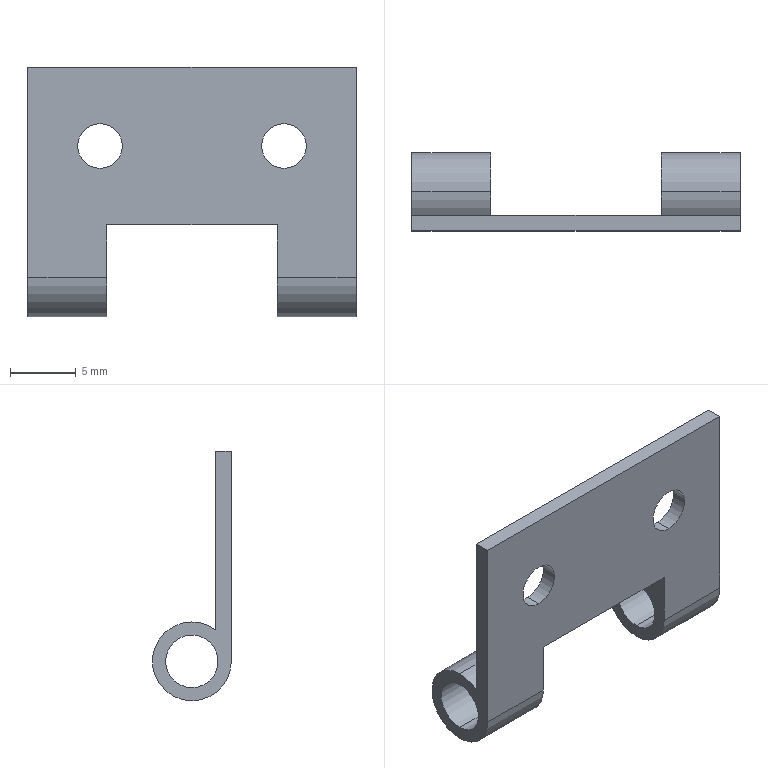Part | SolidWorks | features ICE 2, Extrusion 1 | 1 solid | 22 faces | box 25 x 6 x 19 mm | volume 560.152 mm3 | cylinder 14 | plane 8 | commonest cylinder face diameters 6 x6 3.4 x4 4 x4
STEP:
#1=CARTESIAN_POINT('',(-7.,-3.,8.3));
#2=VERTEX_POINT('',#1);
#3=CARTESIAN_POINT('',(-7.,-3.,11.7));
#4=VERTEX_POINT('',#3);
#5=CARTESIAN_POINT('',(-7.,-3.,10.));
#6=DIRECTION('',(0.,1.,0.));
#7=DIRECTION('',(0.,0.,1.));
#8=AXIS2_PLACEMENT_3D('',#5,#6,#7);
#9=CIRCLE('',#8,1.7);
#10=EDGE_CURVE('',#2,#4,#9,.T.);
#11=ORIENTED_EDGE('',*,*,#10,.F.);
#12=CARTESIAN_POINT('',(-7.,-1.8,8.3));
#13=VERTEX_POINT('',#12);
#14=CARTESIAN_POINT('',(-7.,-3.,8.3));
#15=DIRECTION('',(0.,1.,0.));
#16=VECTOR('',#15,1000.);
#17=LINE('',#14,#16);
#18=EDGE_CURVE('',#2,#13,#17,.T.);
#19=ORIENTED_EDGE('',*,*,#18,.T.);
#20=CARTESIAN_POINT('',(-7.,-1.8,11.7));
#21=VERTEX_POINT('',#20);
#22=CARTESIAN_POINT('',(-7.,-1.8,10.));
#23=DIRECTION('',(0.,1.,0.));
#24=DIRECTION('',(0.,0.,1.));
#25=AXIS2_PLACEMENT_3D('',#22,#23,#24);
#26=CIRCLE('',#25,1.7);
#27=EDGE_CURVE('',#13,#21,#26,.T.);
#28=ORIENTED_EDGE('',*,*,#27,.T.);
#29=CARTESIAN_POINT('',(-7.,-3.,11.7));
#30=DIRECTION('',(0.,1.,0.));
#31=VECTOR('',#30,1000.);
#32=LINE('',#29,#31);
#33=EDGE_CURVE('',#4,#21,#32,.T.);
#34=ORIENTED_EDGE('',*,*,#33,.F.);
#35=EDGE_LOOP('',(#11,#19,#28,#34));
#36=FACE_OUTER_BOUND('',#35,.T.);
#37=CARTESIAN_POINT('',(-7.,-3.,10.));
#38=DIRECTION('',(0.,1.,0.));
#39=DIRECTION('',(0.,0.,1.));
#40=AXIS2_PLACEMENT_3D('',#37,#38,#39);
#41=CYLINDRICAL_SURFACE('',#40,1.7);
#42=ADVANCED_FACE('',(#36),#41,.F.);
#43=CARTESIAN_POINT('',(7.,-3.,8.3));
#44=VERTEX_POINT('',#43);
#45=CARTESIAN_POINT('',(7.,-3.,11.7));
#46=VERTEX_POINT('',#45);
#47=CARTESIAN_POINT('',(7.,-3.,10.));
#48=DIRECTION('',(0.,1.,0.));
#49=DIRECTION('',(0.,0.,1.));
#50=AXIS2_PLACEMENT_3D('',#47,#48,#49);
#51=CIRCLE('',#50,1.7);
#52=EDGE_CURVE('',#44,#46,#51,.T.);
#53=ORIENTED_EDGE('',*,*,#52,.F.);
#54=CARTESIAN_POINT('',(7.,-1.8,8.3));
#55=VERTEX_POINT('',#54);
#56=CARTESIAN_POINT('',(7.,-3.,8.3));
#57=DIRECTION('',(0.,1.,0.));
#58=VECTOR('',#57,1000.);
#59=LINE('',#56,#58);
#60=EDGE_CURVE('',#44,#55,#59,.T.);
#61=ORIENTED_EDGE('',*,*,#60,.T.);
#62=CARTESIAN_POINT('',(7.,-1.8,11.7));
#63=VERTEX_POINT('',#62);
#64=CARTESIAN_POINT('',(7.,-1.8,10.));
#65=DIRECTION('',(0.,1.,0.));
#66=DIRECTION('',(0.,0.,1.));
#67=AXIS2_PLACEMENT_3D('',#64,#65,#66);
#68=CIRCLE('',#67,1.7);
#69=EDGE_CURVE('',#55,#63,#68,.T.);
#70=ORIENTED_EDGE('',*,*,#69,.T.);
#71=CARTESIAN_POINT('',(7.,-3.,11.7));
#72=DIRECTION('',(0.,1.,0.));
#73=VECTOR('',#72,1000.);
#74=LINE('',#71,#73);
#75=EDGE_CURVE('',#46,#63,#74,.T.);
#76=ORIENTED_EDGE('',*,*,#75,.F.);
#77=EDGE_LOOP('',(#53,#61,#70,#76));
#78=FACE_OUTER_BOUND('',#77,.T.);
#79=CARTESIAN_POINT('',(7.,-3.,10.));
#80=DIRECTION('',(0.,1.,0.));
#81=DIRECTION('',(0.,0.,1.));
#82=AXIS2_PLACEMENT_3D('',#79,#80,#81);
#83=CYLINDRICAL_SURFACE('',#82,1.7);
#84=ADVANCED_FACE('',(#78),#83,.F.);
#85=CARTESIAN_POINT('',(12.5,0.,2.));
#86=VERTEX_POINT('',#85);
#87=CARTESIAN_POINT('',(12.5,0.,-2.));
#88=VERTEX_POINT('',#87);
#89=CARTESIAN_POINT('',(12.5,0.,0.));
#90=DIRECTION('',(1.,0.,0.));
#91=DIRECTION('',(0.,0.,-1.));
#92=AXIS2_PLACEMENT_3D('',#89,#90,#91);
#93=CIRCLE('',#92,2.);
#94=EDGE_CURVE('',#86,#88,#93,.T.);
#95=ORIENTED_EDGE('',*,*,#94,.T.);
#96=CARTESIAN_POINT('',(6.5,0.,-2.));
#97=VERTEX_POINT('',#96);
#98=CARTESIAN_POINT('',(12.5,0.,-2.));
#99=DIRECTION('',(-1.,0.,0.));
#100=VECTOR('',#99,1000.);
#101=LINE('',#98,#100);
#102=EDGE_CURVE('',#88,#97,#101,.T.);
#103=ORIENTED_EDGE('',*,*,#102,.T.);
#104=CARTESIAN_POINT('',(6.5,0.,2.));
#105=VERTEX_POINT('',#104);
#106=CARTESIAN_POINT('',(6.5,0.,0.));
#107=DIRECTION('',(1.,0.,0.));
#108=DIRECTION('',(0.,0.,-1.));
#109=AXIS2_PLACEMENT_3D('',#106,#107,#108);
#110=CIRCLE('',#109,2.);
#111=EDGE_CURVE('',#105,#97,#110,.T.);
#112=ORIENTED_EDGE('',*,*,#111,.F.);
#113=CARTESIAN_POINT('',(12.5,0.,2.));
#114=DIRECTION('',(-1.,0.,0.));
#115=VECTOR('',#114,1000.);
#116=LINE('',#113,#115);
#117=EDGE_CURVE('',#86,#105,#116,.T.);
#118=ORIENTED_EDGE('',*,*,#117,.F.);
#119=EDGE_LOOP('',(#95,#103,#112,#118));
#120=FACE_OUTER_BOUND('',#119,.T.);
#121=CARTESIAN_POINT('',(12.5,0.,0.));
#122=DIRECTION('',(-1.,0.,0.));
#123=DIRECTION('',(0.,0.,1.));
#124=AXIS2_PLACEMENT_3D('',#121,#122,#123);
#125=CYLINDRICAL_SURFACE('',#124,2.);
#126=ADVANCED_FACE('',(#120),#125,.F.);
#127=CARTESIAN_POINT('',(12.5,0.,-3.));
#128=VERTEX_POINT('',#127);
#129=CARTESIAN_POINT('',(12.5,0.,3.));
#130=VERTEX_POINT('',#129);
#131=CARTESIAN_POINT('',(12.5,0.,0.));
#132=DIRECTION('',(1.,0.,0.));
#133=DIRECTION('',(0.,0.,-1.));
#134=AXIS2_PLACEMENT_3D('',#131,#132,#133);
#135=CIRCLE('',#134,3.);
#136=EDGE_CURVE('',#128,#130,#135,.T.);
#137=ORIENTED_EDGE('',*,*,#136,.F.);
#138=CARTESIAN_POINT('',(6.5,0.,-3.));
#139=VERTEX_POINT('',#138);
#140=CARTESIAN_POINT('',(12.5,0.,-3.));
#141=DIRECTION('',(-1.,0.,0.));
#142=VECTOR('',#141,1000.);
#143=LINE('',#140,#142);
#144=EDGE_CURVE('',#128,#139,#143,.T.);
#145=ORIENTED_EDGE('',*,*,#144,.T.);
#146=CARTESIAN_POINT('',(6.5,0.,3.));
#147=VERTEX_POINT('',#146);
#148=CARTESIAN_POINT('',(6.5,0.,0.));
#149=DIRECTION('',(1.,0.,0.));
#150=DIRECTION('',(0.,0.,-1.));
#151=AXIS2_PLACEMENT_3D('',#148,#149,#150);
#152=CIRCLE('',#151,3.);
#153=EDGE_CURVE('',#139,#147,#152,.T.);
#154=ORIENTED_EDGE('',*,*,#153,.T.);
#155=CARTESIAN_POINT('',(12.5,0.,3.));
#156=DIRECTION('',(-1.,0.,0.));
#157=VECTOR('',#156,1000.);
#158=LINE('',#155,#157);
#159=EDGE_CURVE('',#130,#147,#158,.T.);
#160=ORIENTED_EDGE('',*,*,#159,.F.);
#161=EDGE_LOOP('',(#137,#145,#154,#160));
#162=FACE_OUTER_BOUND('',#161,.T.);
#163=CARTESIAN_POINT('',(12.5,0.,0.));
#164=DIRECTION('',(-1.,0.,0.));
#165=DIRECTION('',(0.,0.,1.));
#166=AXIS2_PLACEMENT_3D('',#163,#164,#165);
#167=CYLINDRICAL_SURFACE('',#166,3.);
#168=ADVANCED_FACE('',(#162),#167,.T.);
#169=CARTESIAN_POINT('',(12.5,-1.8,2.4));
#170=VERTEX_POINT('',#169);
#171=CARTESIAN_POINT('',(12.5,0.,0.));
#172=DIRECTION('',(1.,0.,0.));
#173=DIRECTION('',(0.,0.,-1.));
#174=AXIS2_PLACEMENT_3D('',#171,#172,#173);
#175=CIRCLE('',#174,3.);
#176=EDGE_CURVE('',#130,#170,#175,.T.);
#177=ORIENTED_EDGE('',*,*,#176,.F.);
#178=ORIENTED_EDGE('',*,*,#159,.T.);
#179=CARTESIAN_POINT('',(6.5,-1.8,2.4));
#180=VERTEX_POINT('',#179);
#181=CARTESIAN_POINT('',(6.5,0.,0.));
#182=DIRECTION('',(1.,0.,0.));
#183=DIRECTION('',(0.,0.,-1.));
#184=AXIS2_PLACEMENT_3D('',#181,#182,#183);
#185=CIRCLE('',#184,3.);
#186=EDGE_CURVE('',#147,#180,#185,.T.);
#187=ORIENTED_EDGE('',*,*,#186,.T.);
#188=CARTESIAN_POINT('',(12.5,-1.8,2.4));
#189=DIRECTION('',(-1.,0.,0.));
#190=VECTOR('',#189,1000.);
#191=LINE('',#188,#190);
#192=EDGE_CURVE('',#170,#180,#191,.T.);
#193=ORIENTED_EDGE('',*,*,#192,.F.);
#194=EDGE_LOOP('',(#177,#178,#187,#193));
#195=FACE_OUTER_BOUND('',#194,.T.);
#196=CARTESIAN_POINT('',(12.5,0.,0.));
#197=DIRECTION('',(-1.,0.,0.));
#198=DIRECTION('',(0.,0.,1.));
#199=AXIS2_PLACEMENT_3D('',#196,#197,#198);
#200=CYLINDRICAL_SURFACE('',#199,3.);
#201=ADVANCED_FACE('',(#195),#200,.T.);
#202=CARTESIAN_POINT('',(-6.5,0.,2.));
#203=VERTEX_POINT('',#202);
#204=CARTESIAN_POINT('',(-6.5,0.,-2.));
#205=VERTEX_POINT('',#204);
#206=CARTESIAN_POINT('',(-6.5,0.,0.));
#207=DIRECTION('',(1.,0.,0.));
#208=DIRECTION('',(0.,0.,-1.));
#209=AXIS2_PLACEMENT_3D('',#206,#207,#208);
#210=CIRCLE('',#209,2.);
#211=EDGE_CURVE('',#203,#205,#210,.T.);
#212=ORIENTED_EDGE('',*,*,#211,.T.);
#213=CARTESIAN_POINT('',(-12.5,0.,-2.));
#214=VERTEX_POINT('',#213);
#215=CARTESIAN_POINT('',(12.5,0.,-2.));
#216=DIRECTION('',(-1.,0.,0.));
#217=VECTOR('',#216,1000.);
#218=LINE('',#215,#217);
#219=EDGE_CURVE('',#205,#214,#218,.T.);
#220=ORIENTED_EDGE('',*,*,#219,.T.);
#221=CARTESIAN_POINT('',(-12.5,0.,2.));
#222=VERTEX_POINT('',#221);
#223=CARTESIAN_POINT('',(-12.5,0.,0.));
#224=DIRECTION('',(1.,0.,0.));
#225=DIRECTION('',(0.,0.,-1.));
#226=AXIS2_PLACEMENT_3D('',#223,#224,#225);
#227=CIRCLE('',#226,2.);
#228=EDGE_CURVE('',#222,#214,#227,.T.);
#229=ORIENTED_EDGE('',*,*,#228,.F.);
#230=CARTESIAN_POINT('',(12.5,0.,2.));
#231=DIRECTION('',(-1.,0.,0.));
#232=VECTOR('',#231,1000.);
#233=LINE('',#230,#232);
#234=EDGE_CURVE('',#203,#222,#233,.T.);
#235=ORIENTED_EDGE('',*,*,#234,.F.);
#236=EDGE_LOOP('',(#212,#220,#229,#235));
#237=FACE_OUTER_BOUND('',#236,.T.);
#238=CARTESIAN_POINT('',(12.5,0.,0.));
#239=DIRECTION('',(-1.,0.,0.));
#240=DIRECTION('',(0.,0.,1.));
#241=AXIS2_PLACEMENT_3D('',#238,#239,#240);
#242=CYLINDRICAL_SURFACE('',#241,2.);
#243=ADVANCED_FACE('',(#237),#242,.F.);
#244=CARTESIAN_POINT('',(-6.5,0.,-3.));
#245=VERTEX_POINT('',#244);
#246=CARTESIAN_POINT('',(-6.5,0.,3.));
#247=VERTEX_POINT('',#246);
#248=CARTESIAN_POINT('',(-6.5,0.,0.));
#249=DIRECTION('',(1.,0.,0.));
#250=DIRECTION('',(0.,0.,-1.));
#251=AXIS2_PLACEMENT_3D('',#248,#249,#250);
#252=CIRCLE('',#251,3.);
#253=EDGE_CURVE('',#245,#247,#252,.T.);
#254=ORIENTED_EDGE('',*,*,#253,.F.);
#255=CARTESIAN_POINT('',(-12.5,0.,-3.));
#256=VERTEX_POINT('',#255);
#257=CARTESIAN_POINT('',(12.5,0.,-3.));
#258=DIRECTION('',(-1.,0.,0.));
#259=VECTOR('',#258,1000.);
#260=LINE('',#257,#259);
#261=EDGE_CURVE('',#245,#256,#260,.T.);
#262=ORIENTED_EDGE('',*,*,#261,.T.);
#263=CARTESIAN_POINT('',(-12.5,0.,3.));
#264=VERTEX_POINT('',#263);
#265=CARTESIAN_POINT('',(-12.5,0.,0.));
#266=DIRECTION('',(1.,0.,0.));
#267=DIRECTION('',(0.,0.,-1.));
#268=AXIS2_PLACEMENT_3D('',#265,#266,#267);
#269=CIRCLE('',#268,3.);
#270=EDGE_CURVE('',#256,#264,#269,.T.);
#271=ORIENTED_EDGE('',*,*,#270,.T.);
#272=CARTESIAN_POINT('',(12.5,0.,3.));
#273=DIRECTION('',(-1.,0.,0.));
#274=VECTOR('',#273,1000.);
#275=LINE('',#272,#274);
#276=EDGE_CURVE('',#247,#264,#275,.T.);
#277=ORIENTED_EDGE('',*,*,#276,.F.);
#278=EDGE_LOOP('',(#254,#262,#271,#277));
#279=FACE_OUTER_BOUND('',#278,.T.);
#280=CARTESIAN_POINT('',(12.5,0.,0.));
#281=DIRECTION('',(-1.,0.,0.));
#282=DIRECTION('',(0.,0.,1.));
#283=AXIS2_PLACEMENT_3D('',#280,#281,#282);
#284=CYLINDRICAL_SURFACE('',#283,3.);
#285=ADVANCED_FACE('',(#279),#284,.T.);
#286=CARTESIAN_POINT('',(-6.5,-1.8,2.4));
#287=VERTEX_POINT('',#286);
#288=CARTESIAN_POINT('',(-6.5,0.,0.));
#289=DIRECTION('',(1.,0.,0.));
#290=DIRECTION('',(0.,0.,-1.));
#291=AXIS2_PLACEMENT_3D('',#288,#289,#290);
#292=CIRCLE('',#291,3.);
#293=EDGE_CURVE('',#247,#287,#292,.T.);
#294=ORIENTED_EDGE('',*,*,#293,.F.);
#295=ORIENTED_EDGE('',*,*,#276,.T.);
#296=CARTESIAN_POINT('',(-12.5,-1.8,2.4));
#297=VERTEX_POINT('',#296);
#298=CARTESIAN_POINT('',(-12.5,0.,0.));
#299=DIRECTION('',(1.,0.,0.));
#300=DIRECTION('',(0.,0.,-1.));
#301=AXIS2_PLACEMENT_3D('',#298,#299,#300);
#302=CIRCLE('',#301,3.);
#303=EDGE_CURVE('',#264,#297,#302,.T.);
#304=ORIENTED_EDGE('',*,*,#303,.T.);
#305=CARTESIAN_POINT('',(12.5,-1.8,2.4));
#306=DIRECTION('',(-1.,0.,0.));
#307=VECTOR('',#306,1000.);
#308=LINE('',#305,#307);
#309=EDGE_CURVE('',#287,#297,#308,.T.);
#310=ORIENTED_EDGE('',*,*,#309,.F.);
#311=EDGE_LOOP('',(#294,#295,#304,#310));
#312=FACE_OUTER_BOUND('',#311,.T.);
#313=CARTESIAN_POINT('',(12.5,0.,0.));
#314=DIRECTION('',(-1.,0.,0.));
#315=DIRECTION('',(0.,0.,1.));
#316=AXIS2_PLACEMENT_3D('',#313,#314,#315);
#317=CYLINDRICAL_SURFACE('',#316,3.);
#318=ADVANCED_FACE('',(#312),#317,.T.);
#319=ORIENTED_EDGE('',*,*,#261,.F.);
#320=CARTESIAN_POINT('',(-6.5,-3.,0.));
#321=VERTEX_POINT('',#320);
#322=CARTESIAN_POINT('',(-6.5,0.,0.));
#323=DIRECTION('',(1.,0.,0.));
#324=DIRECTION('',(0.,0.,-1.));
#325=AXIS2_PLACEMENT_3D('',#322,#323,#324);
#326=CIRCLE('',#325,3.);
#327=EDGE_CURVE('',#321,#245,#326,.T.);
#328=ORIENTED_EDGE('',*,*,#327,.F.);
#329=CARTESIAN_POINT('',(-12.5,-3.,0.));
#330=VERTEX_POINT('',#329);
#331=CARTESIAN_POINT('',(12.5,-3.,0.));
#332=DIRECTION('',(-1.,0.,0.));
#333=VECTOR('',#332,1000.);
#334=LINE('',#331,#333);
#335=EDGE_CURVE('',#321,#330,#334,.T.);
#336=ORIENTED_EDGE('',*,*,#335,.T.);
#337=CARTESIAN_POINT('',(-12.5,0.,0.));
#338=DIRECTION('',(1.,0.,0.));
#339=DIRECTION('',(0.,0.,-1.));
#340=AXIS2_PLACEMENT_3D('',#337,#338,#339);
#341=CIRCLE('',#340,3.);
#342=EDGE_CURVE('',#330,#256,#341,.T.);
#343=ORIENTED_EDGE('',*,*,#342,.T.);
#344=EDGE_LOOP('',(#319,#328,#336,#343));
#345=FACE_OUTER_BOUND('',#344,.T.);
#346=CARTESIAN_POINT('',(12.5,0.,0.));
#347=DIRECTION('',(-1.,0.,0.));
#348=DIRECTION('',(0.,0.,1.));
#349=AXIS2_PLACEMENT_3D('',#346,#347,#348);
#350=CYLINDRICAL_SURFACE('',#349,3.);
#351=ADVANCED_FACE('',(#345),#350,.T.);
#352=CARTESIAN_POINT('',(7.,-1.8,10.));
#353=DIRECTION('',(0.,1.,0.));
#354=DIRECTION('',(0.,0.,1.));
#355=AXIS2_PLACEMENT_3D('',#352,#353,#354);
#356=CIRCLE('',#355,1.7);
#357=EDGE_CURVE('',#63,#55,#356,.T.);
#358=ORIENTED_EDGE('',*,*,#357,.F.);
#359=ORIENTED_EDGE('',*,*,#69,.F.);
#360=EDGE_LOOP('',(#358,#359));
#361=FACE_BOUND('',#360,.T.);
#362=CARTESIAN_POINT('',(-7.,-1.8,10.));
#363=DIRECTION('',(0.,1.,0.));
#364=DIRECTION('',(0.,0.,1.));
#365=AXIS2_PLACEMENT_3D('',#362,#363,#364);
#366=CIRCLE('',#365,1.7);
#367=EDGE_CURVE('',#21,#13,#366,.T.);
#368=ORIENTED_EDGE('',*,*,#367,.F.);
#369=ORIENTED_EDGE('',*,*,#27,.F.);
#370=EDGE_LOOP('',(#368,#369));
#371=FACE_BOUND('',#370,.T.);
#372=CARTESIAN_POINT('',(-6.5,-1.8,4.));
#373=VERTEX_POINT('',#372);
#374=CARTESIAN_POINT('',(-6.5,-1.8,2.4));
#375=DIRECTION('',(0.,0.,1.));
#376=VECTOR('',#375,1000.);
#377=LINE('',#374,#376);
#378=EDGE_CURVE('',#287,#373,#377,.T.);
#379=ORIENTED_EDGE('',*,*,#378,.F.);
#380=ORIENTED_EDGE('',*,*,#309,.T.);
#381=CARTESIAN_POINT('',(-12.5,-1.8,16.));
#382=VERTEX_POINT('',#381);
#383=CARTESIAN_POINT('',(-12.5,-1.8,16.));
#384=DIRECTION('',(0.,0.,1.));
#385=VECTOR('',#384,1000.);
#386=LINE('',#383,#385);
#387=EDGE_CURVE('',#297,#382,#386,.T.);
#388=ORIENTED_EDGE('',*,*,#387,.T.);
#389=CARTESIAN_POINT('',(12.5,-1.8,16.));
#390=VERTEX_POINT('',#389);
#391=CARTESIAN_POINT('',(12.5,-1.8,16.));
#392=DIRECTION('',(-1.,0.,0.));
#393=VECTOR('',#392,1000.);
#394=LINE('',#391,#393);
#395=EDGE_CURVE('',#390,#382,#394,.T.);
#396=ORIENTED_EDGE('',*,*,#395,.F.);
#397=CARTESIAN_POINT('',(12.5,-1.8,16.));
#398=DIRECTION('',(0.,0.,1.));
#399=VECTOR('',#398,1000.);
#400=LINE('',#397,#399);
#401=EDGE_CURVE('',#170,#390,#400,.T.);
#402=ORIENTED_EDGE('',*,*,#401,.F.);
#403=ORIENTED_EDGE('',*,*,#192,.T.);
#404=CARTESIAN_POINT('',(6.5,-1.8,4.));
#405=VERTEX_POINT('',#404);
#406=CARTESIAN_POINT('',(6.5,-1.8,2.4));
#407=DIRECTION('',(0.,0.,1.));
#408=VECTOR('',#407,1000.);
#409=LINE('',#406,#408);
#410=EDGE_CURVE('',#180,#405,#409,.T.);
#411=ORIENTED_EDGE('',*,*,#410,.T.);
#412=CARTESIAN_POINT('',(-6.5,-1.8,4.));
#413=DIRECTION('',(1.,0.,0.));
#414=VECTOR('',#413,1000.);
#415=LINE('',#412,#414);
#416=EDGE_CURVE('',#373,#405,#415,.T.);
#417=ORIENTED_EDGE('',*,*,#416,.F.);
#418=EDGE_LOOP('',(#379,#380,#388,#396,#402,#403,#411,#417));
#419=FACE_OUTER_BOUND('',#418,.T.);
#420=CARTESIAN_POINT('',(12.5,-1.8,16.));
#421=DIRECTION('',(0.,-1.,0.));
#422=DIRECTION('',(0.,0.,-1.));
#423=AXIS2_PLACEMENT_3D('',#420,#421,#422);
#424=PLANE('',#423);
#425=ADVANCED_FACE('',(#361,#371,#419),#424,.F.);
#426=CARTESIAN_POINT('',(7.,-3.,10.));
#427=DIRECTION('',(0.,1.,0.));
#428=DIRECTION('',(0.,0.,1.));
#429=AXIS2_PLACEMENT_3D('',#426,#427,#428);
#430=CIRCLE('',#429,1.7);
#431=EDGE_CURVE('',#46,#44,#430,.T.);
#432=ORIENTED_EDGE('',*,*,#431,.T.);
#433=ORIENTED_EDGE('',*,*,#52,.T.);
#434=EDGE_LOOP('',(#432,#433));
#435=FACE_BOUND('',#434,.T.);
#436=CARTESIAN_POINT('',(-7.,-3.,10.));
#437=DIRECTION('',(0.,1.,0.));
#438=DIRECTION('',(0.,0.,1.));
#439=AXIS2_PLACEMENT_3D('',#436,#437,#438);
#440=CIRCLE('',#439,1.7);
#441=EDGE_CURVE('',#4,#2,#440,.T.);
#442=ORIENTED_EDGE('',*,*,#441,.T.);
#443=ORIENTED_EDGE('',*,*,#10,.T.);
#444=EDGE_LOOP('',(#442,#443));
#445=FACE_BOUND('',#444,.T.);
#446=CARTESIAN_POINT('',(-6.5,-3.,4.));
#447=VERTEX_POINT('',#446);
#448=CARTESIAN_POINT('',(-6.5,-3.,4.));
#449=DIRECTION('',(0.,0.,-1.));
#450=VECTOR('',#449,1000.);
#451=LINE('',#448,#450);
#452=EDGE_CURVE('',#447,#321,#451,.T.);
#453=ORIENTED_EDGE('',*,*,#452,.F.);
#454=CARTESIAN_POINT('',(6.5,-3.,4.));
#455=VERTEX_POINT('',#454);
#456=CARTESIAN_POINT('',(-6.5,-3.,4.));
#457=DIRECTION('',(1.,0.,0.));
#458=VECTOR('',#457,1000.);
#459=LINE('',#456,#458);
#460=EDGE_CURVE('',#447,#455,#459,.T.);
#461=ORIENTED_EDGE('',*,*,#460,.T.);
#462=CARTESIAN_POINT('',(6.5,-3.,0.));
#463=VERTEX_POINT('',#462);
#464=CARTESIAN_POINT('',(6.5,-3.,4.));
#465=DIRECTION('',(0.,0.,-1.));
#466=VECTOR('',#465,1000.);
#467=LINE('',#464,#466);
#468=EDGE_CURVE('',#455,#463,#467,.T.);
#469=ORIENTED_EDGE('',*,*,#468,.T.);
#470=CARTESIAN_POINT('',(12.5,-3.,0.));
#471=VERTEX_POINT('',#470);
#472=CARTESIAN_POINT('',(12.5,-3.,0.));
#473=DIRECTION('',(-1.,0.,0.));
#474=VECTOR('',#473,1000.);
#475=LINE('',#472,#474);
#476=EDGE_CURVE('',#471,#463,#475,.T.);
#477=ORIENTED_EDGE('',*,*,#476,.F.);
#478=CARTESIAN_POINT('',(12.5,-3.,16.));
#479=VERTEX_POINT('',#478);
#480=CARTESIAN_POINT('',(12.5,-3.,0.));
#481=DIRECTION('',(0.,0.,-1.));
#482=VECTOR('',#481,1000.);
#483=LINE('',#480,#482);
#484=EDGE_CURVE('',#479,#471,#483,.T.);
#485=ORIENTED_EDGE('',*,*,#484,.F.);
#486=CARTESIAN_POINT('',(-12.5,-3.,16.));
#487=VERTEX_POINT('',#486);
#488=CARTESIAN_POINT('',(12.5,-3.,16.));
#489=DIRECTION('',(-1.,0.,0.));
#490=VECTOR('',#489,1000.);
#491=LINE('',#488,#490);
#492=EDGE_CURVE('',#479,#487,#491,.T.);
#493=ORIENTED_EDGE('',*,*,#492,.T.);
#494=CARTESIAN_POINT('',(-12.5,-3.,0.));
#495=DIRECTION('',(0.,0.,-1.));
#496=VECTOR('',#495,1000.);
#497=LINE('',#494,#496);
#498=EDGE_CURVE('',#487,#330,#497,.T.);
#499=ORIENTED_EDGE('',*,*,#498,.T.);
#500=ORIENTED_EDGE('',*,*,#335,.F.);
#501=EDGE_LOOP('',(#453,#461,#469,#477,#485,#493,#499,#500));
#502=FACE_OUTER_BOUND('',#501,.T.);
#503=CARTESIAN_POINT('',(12.5,-3.,0.));
#504=DIRECTION('',(0.,1.,0.));
#505=DIRECTION('',(0.,0.,1.));
#506=AXIS2_PLACEMENT_3D('',#503,#504,#505);
#507=PLANE('',#506);
#508=ADVANCED_FACE('',(#435,#445,#502),#507,.F.);
#509=ORIENTED_EDGE('',*,*,#219,.F.);
#510=CARTESIAN_POINT('',(-6.5,0.,0.));
#511=DIRECTION('',(1.,0.,0.));
#512=DIRECTION('',(0.,0.,-1.));
#513=AXIS2_PLACEMENT_3D('',#510,#511,#512);
#514=CIRCLE('',#513,2.);
#515=EDGE_CURVE('',#205,#203,#514,.T.);
#516=ORIENTED_EDGE('',*,*,#515,.T.);
#517=ORIENTED_EDGE('',*,*,#234,.T.);
#518=CARTESIAN_POINT('',(-12.5,0.,0.));
#519=DIRECTION('',(1.,0.,0.));
#520=DIRECTION('',(0.,0.,-1.));
#521=AXIS2_PLACEMENT_3D('',#518,#519,#520);
#522=CIRCLE('',#521,2.);
#523=EDGE_CURVE('',#214,#222,#522,.T.);
#524=ORIENTED_EDGE('',*,*,#523,.F.);
#525=EDGE_LOOP('',(#509,#516,#517,#524));
#526=FACE_OUTER_BOUND('',#525,.T.);
#527=CARTESIAN_POINT('',(12.5,0.,0.));
#528=DIRECTION('',(-1.,0.,0.));
#529=DIRECTION('',(0.,0.,1.));
#530=AXIS2_PLACEMENT_3D('',#527,#528,#529);
#531=CYLINDRICAL_SURFACE('',#530,2.);
#532=ADVANCED_FACE('',(#526),#531,.F.);
#533=CARTESIAN_POINT('',(12.5,0.,0.));
#534=DIRECTION('',(1.,0.,0.));
#535=DIRECTION('',(0.,0.,-1.));
#536=AXIS2_PLACEMENT_3D('',#533,#534,#535);
#537=CIRCLE('',#536,3.);
#538=EDGE_CURVE('',#471,#128,#537,.T.);
#539=ORIENTED_EDGE('',*,*,#538,.T.);
#540=ORIENTED_EDGE('',*,*,#136,.T.);
#541=ORIENTED_EDGE('',*,*,#176,.T.);
#542=ORIENTED_EDGE('',*,*,#401,.T.);
#543=CARTESIAN_POINT('',(12.5,-3.,16.));
#544=DIRECTION('',(0.,-1.,0.));
#545=VECTOR('',#544,1000.);
#546=LINE('',#543,#545);
#547=EDGE_CURVE('',#390,#479,#546,.T.);
#548=ORIENTED_EDGE('',*,*,#547,.T.);
#549=ORIENTED_EDGE('',*,*,#484,.T.);
#550=EDGE_LOOP('',(#539,#540,#541,#542,#548,#549));
#551=FACE_OUTER_BOUND('',#550,.T.);
#552=ORIENTED_EDGE('',*,*,#94,.F.);
#553=CARTESIAN_POINT('',(12.5,0.,0.));
#554=DIRECTION('',(1.,0.,0.));
#555=DIRECTION('',(0.,0.,-1.));
#556=AXIS2_PLACEMENT_3D('',#553,#554,#555);
#557=CIRCLE('',#556,2.);
#558=EDGE_CURVE('',#88,#86,#557,.T.);
#559=ORIENTED_EDGE('',*,*,#558,.F.);
#560=EDGE_LOOP('',(#552,#559));
#561=FACE_BOUND('',#560,.T.);
#562=CARTESIAN_POINT('',(12.5,0.,0.));
#563=DIRECTION('',(1.,0.,0.));
#564=DIRECTION('',(0.,0.,-1.));
#565=AXIS2_PLACEMENT_3D('',#562,#563,#564);
#566=PLANE('',#565);
#567=ADVANCED_FACE('',(#551,#561),#566,.T.);
#568=ORIENTED_EDGE('',*,*,#342,.F.);
#569=ORIENTED_EDGE('',*,*,#498,.F.);
#570=CARTESIAN_POINT('',(-12.5,-3.,16.));
#571=DIRECTION('',(0.,-1.,0.));
#572=VECTOR('',#571,1000.);
#573=LINE('',#570,#572);
#574=EDGE_CURVE('',#382,#487,#573,.T.);
#575=ORIENTED_EDGE('',*,*,#574,.F.);
#576=ORIENTED_EDGE('',*,*,#387,.F.);
#577=ORIENTED_EDGE('',*,*,#303,.F.);
#578=ORIENTED_EDGE('',*,*,#270,.F.);
#579=EDGE_LOOP('',(#568,#569,#575,#576,#577,#578));
#580=FACE_OUTER_BOUND('',#579,.T.);
#581=ORIENTED_EDGE('',*,*,#228,.T.);
#582=ORIENTED_EDGE('',*,*,#523,.T.);
#583=EDGE_LOOP('',(#581,#582));
#584=FACE_BOUND('',#583,.T.);
#585=CARTESIAN_POINT('',(-12.5,0.,0.));
#586=DIRECTION('',(1.,0.,0.));
#587=DIRECTION('',(0.,0.,-1.));
#588=AXIS2_PLACEMENT_3D('',#585,#586,#587);
#589=PLANE('',#588);
#590=ADVANCED_FACE('',(#580,#584),#589,.F.);
#591=ORIENTED_EDGE('',*,*,#144,.F.);
#592=ORIENTED_EDGE('',*,*,#538,.F.);
#593=ORIENTED_EDGE('',*,*,#476,.T.);
#594=CARTESIAN_POINT('',(6.5,0.,0.));
#595=DIRECTION('',(1.,0.,0.));
#596=DIRECTION('',(0.,0.,-1.));
#597=AXIS2_PLACEMENT_3D('',#594,#595,#596);
#598=CIRCLE('',#597,3.);
#599=EDGE_CURVE('',#463,#139,#598,.T.);
#600=ORIENTED_EDGE('',*,*,#599,.T.);
#601=EDGE_LOOP('',(#591,#592,#593,#600));
#602=FACE_OUTER_BOUND('',#601,.T.);
#603=CARTESIAN_POINT('',(12.5,0.,0.));
#604=DIRECTION('',(-1.,0.,0.));
#605=DIRECTION('',(0.,0.,1.));
#606=AXIS2_PLACEMENT_3D('',#603,#604,#605);
#607=CYLINDRICAL_SURFACE('',#606,3.);
#608=ADVANCED_FACE('',(#602),#607,.T.);
#609=ORIENTED_EDGE('',*,*,#574,.T.);
#610=ORIENTED_EDGE('',*,*,#492,.F.);
#611=ORIENTED_EDGE('',*,*,#547,.F.);
#612=ORIENTED_EDGE('',*,*,#395,.T.);
#613=EDGE_LOOP('',(#609,#610,#611,#612));
#614=FACE_OUTER_BOUND('',#613,.T.);
#615=CARTESIAN_POINT('',(12.5,-3.,16.));
#616=DIRECTION('',(0.,0.,-1.));
#617=DIRECTION('',(-1.,0.,0.));
#618=AXIS2_PLACEMENT_3D('',#615,#616,#617);
#619=PLANE('',#618);
#620=ADVANCED_FACE('',(#614),#619,.F.);
#621=ORIENTED_EDGE('',*,*,#102,.F.);
#622=ORIENTED_EDGE('',*,*,#558,.T.);
#623=ORIENTED_EDGE('',*,*,#117,.T.);
#624=CARTESIAN_POINT('',(6.5,0.,0.));
#625=DIRECTION('',(1.,0.,0.));
#626=DIRECTION('',(0.,0.,-1.));
#627=AXIS2_PLACEMENT_3D('',#624,#625,#626);
#628=CIRCLE('',#627,2.);
#629=EDGE_CURVE('',#97,#105,#628,.T.);
#630=ORIENTED_EDGE('',*,*,#629,.F.);
#631=EDGE_LOOP('',(#621,#622,#623,#630));
#632=FACE_OUTER_BOUND('',#631,.T.);
#633=CARTESIAN_POINT('',(12.5,0.,0.));
#634=DIRECTION('',(-1.,0.,0.));
#635=DIRECTION('',(0.,0.,1.));
#636=AXIS2_PLACEMENT_3D('',#633,#634,#635);
#637=CYLINDRICAL_SURFACE('',#636,2.);
#638=ADVANCED_FACE('',(#632),#637,.F.);
#639=ORIENTED_EDGE('',*,*,#60,.F.);
#640=ORIENTED_EDGE('',*,*,#431,.F.);
#641=ORIENTED_EDGE('',*,*,#75,.T.);
#642=ORIENTED_EDGE('',*,*,#357,.T.);
#643=EDGE_LOOP('',(#639,#640,#641,#642));
#644=FACE_OUTER_BOUND('',#643,.T.);
#645=CARTESIAN_POINT('',(7.,-3.,10.));
#646=DIRECTION('',(0.,1.,0.));
#647=DIRECTION('',(0.,0.,1.));
#648=AXIS2_PLACEMENT_3D('',#645,#646,#647);
#649=CYLINDRICAL_SURFACE('',#648,1.7);
#650=ADVANCED_FACE('',(#644),#649,.F.);
#651=ORIENTED_EDGE('',*,*,#18,.F.);
#652=ORIENTED_EDGE('',*,*,#441,.F.);
#653=ORIENTED_EDGE('',*,*,#33,.T.);
#654=ORIENTED_EDGE('',*,*,#367,.T.);
#655=EDGE_LOOP('',(#651,#652,#653,#654));
#656=FACE_OUTER_BOUND('',#655,.T.);
#657=CARTESIAN_POINT('',(-7.,-3.,10.));
#658=DIRECTION('',(0.,1.,0.));
#659=DIRECTION('',(0.,0.,1.));
#660=AXIS2_PLACEMENT_3D('',#657,#658,#659);
#661=CYLINDRICAL_SURFACE('',#660,1.7);
#662=ADVANCED_FACE('',(#656),#661,.F.);
#663=CARTESIAN_POINT('',(6.5,-1.8,4.));
#664=DIRECTION('',(0.,-1.,0.));
#665=VECTOR('',#664,1000.);
#666=LINE('',#663,#665);
#667=EDGE_CURVE('',#405,#455,#666,.T.);
#668=ORIENTED_EDGE('',*,*,#667,.T.);
#669=ORIENTED_EDGE('',*,*,#460,.F.);
#670=CARTESIAN_POINT('',(-6.5,-1.8,4.));
#671=DIRECTION('',(0.,-1.,0.));
#672=VECTOR('',#671,1000.);
#673=LINE('',#670,#672);
#674=EDGE_CURVE('',#373,#447,#673,.T.);
#675=ORIENTED_EDGE('',*,*,#674,.F.);
#676=ORIENTED_EDGE('',*,*,#416,.T.);
#677=EDGE_LOOP('',(#668,#669,#675,#676));
#678=FACE_OUTER_BOUND('',#677,.T.);
#679=CARTESIAN_POINT('',(-6.5,-1.8,4.));
#680=DIRECTION('',(0.,0.,1.));
#681=DIRECTION('',(1.,0.,0.));
#682=AXIS2_PLACEMENT_3D('',#679,#680,#681);
#683=PLANE('',#682);
#684=ADVANCED_FACE('',(#678),#683,.F.);
#685=ORIENTED_EDGE('',*,*,#211,.F.);
#686=ORIENTED_EDGE('',*,*,#515,.F.);
#687=EDGE_LOOP('',(#685,#686));
#688=FACE_BOUND('',#687,.T.);
#689=ORIENTED_EDGE('',*,*,#327,.T.);
#690=ORIENTED_EDGE('',*,*,#253,.T.);
#691=ORIENTED_EDGE('',*,*,#293,.T.);
#692=ORIENTED_EDGE('',*,*,#378,.T.);
#693=ORIENTED_EDGE('',*,*,#674,.T.);
#694=ORIENTED_EDGE('',*,*,#452,.T.);
#695=EDGE_LOOP('',(#689,#690,#691,#692,#693,#694));
#696=FACE_OUTER_BOUND('',#695,.T.);
#697=CARTESIAN_POINT('',(-6.5,0.,0.));
#698=DIRECTION('',(1.,0.,0.));
#699=DIRECTION('',(0.,0.,-1.));
#700=AXIS2_PLACEMENT_3D('',#697,#698,#699);
#701=PLANE('',#700);
#702=ADVANCED_FACE('',(#688,#696),#701,.T.);
#703=ORIENTED_EDGE('',*,*,#111,.T.);
#704=ORIENTED_EDGE('',*,*,#629,.T.);
#705=EDGE_LOOP('',(#703,#704));
#706=FACE_BOUND('',#705,.T.);
#707=ORIENTED_EDGE('',*,*,#599,.F.);
#708=ORIENTED_EDGE('',*,*,#468,.F.);
#709=ORIENTED_EDGE('',*,*,#667,.F.);
#710=ORIENTED_EDGE('',*,*,#410,.F.);
#711=ORIENTED_EDGE('',*,*,#186,.F.);
#712=ORIENTED_EDGE('',*,*,#153,.F.);
#713=EDGE_LOOP('',(#707,#708,#709,#710,#711,#712));
#714=FACE_OUTER_BOUND('',#713,.T.);
#715=CARTESIAN_POINT('',(6.5,0.,0.));
#716=DIRECTION('',(1.,0.,0.));
#717=DIRECTION('',(0.,0.,-1.));
#718=AXIS2_PLACEMENT_3D('',#715,#716,#717);
#719=PLANE('',#718);
#720=ADVANCED_FACE('',(#706,#714),#719,.F.);
#721=CLOSED_SHELL('',(#42,#84,#126,#168,#201,#243,#285,#318,#351,#425,#508,#532,#567,#590,#608,#620,#638,#650,#662,#684,#702,#720));
#722=MANIFOLD_SOLID_BREP('',#721);
#723=CARTESIAN_POINT('',(0.,0.,0.));
#724=DIRECTION('',(0.,0.,1.));
#725=DIRECTION('',(1.,0.,0.));
#726=AXIS2_PLACEMENT_3D('',#723,#724,#725);
#727=(LENGTH_UNIT()NAMED_UNIT(*)SI_UNIT(.MILLI.,.METRE.));
#728=UNCERTAINTY_MEASURE_WITH_UNIT(LENGTH_MEASURE(0.00001),#727,'','');
#729=(NAMED_UNIT(*)PLANE_ANGLE_UNIT()SI_UNIT($,.RADIAN.));
#730=(NAMED_UNIT(*)SI_UNIT($,.STERADIAN.)SOLID_ANGLE_UNIT());
#731=(GEOMETRIC_REPRESENTATION_CONTEXT(3)GLOBAL_UNCERTAINTY_ASSIGNED_CONTEXT((#728))GLOBAL_UNIT_ASSIGNED_CONTEXT((#727,#729,#730))REPRESENTATION_CONTEXT('',''));
#732=ADVANCED_BREP_SHAPE_REPRESENTATION('',(#722,#726),#731);